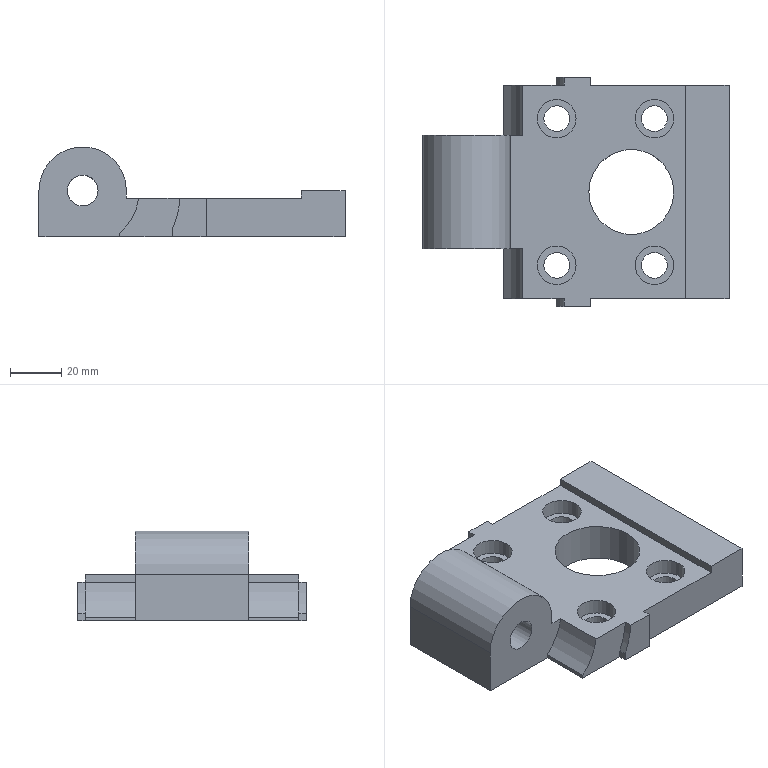Part | NX | features EXTRUDE 11, CBORE_HOLE 4, DATUM_CSYS 4, SKETCH 3, HOLE PACKAGE 1 | 1 solid | 40 faces | box 119 x 89 x 35 mm | volume 132113 mm3 | plane 25 | cylinder 15 | commonest cylinder face diameters 10 x4 15 x4 44 x2 76 x2 12 x1 33 x1
STEP:
#1=CARTESIAN_POINT('',(51.049,70.,15.));
#2=VERTEX_POINT('',#1);
#3=CARTESIAN_POINT('',(58.549,70.,15.));
#4=DIRECTION('',(0.,0.,-1.));
#5=DIRECTION('',(-1.,0.,0.));
#6=AXIS2_PLACEMENT_3D('',#3,#4,#5);
#7=CIRCLE('',#6,7.5);
#8=EDGE_CURVE('',#2,#2,#7,.T.);
#9=ORIENTED_EDGE('',*,*,#8,.T.);
#10=EDGE_LOOP('',(#9));
#11=FACE_BOUND('',#10,.T.);
#12=CARTESIAN_POINT('',(51.049,13.,15.));
#13=VERTEX_POINT('',#12);
#14=CARTESIAN_POINT('',(58.549,13.,15.));
#15=DIRECTION('',(0.,0.,-1.));
#16=DIRECTION('',(-1.,0.,0.));
#17=AXIS2_PLACEMENT_3D('',#14,#15,#16);
#18=CIRCLE('',#17,7.5);
#19=EDGE_CURVE('',#13,#13,#18,.T.);
#20=ORIENTED_EDGE('',*,*,#19,.T.);
#21=EDGE_LOOP('',(#20));
#22=FACE_BOUND('',#21,.T.);
#23=CARTESIAN_POINT('',(13.049,70.,15.));
#24=VERTEX_POINT('',#23);
#25=CARTESIAN_POINT('',(20.549,70.,15.));
#26=DIRECTION('',(0.,0.,-1.));
#27=DIRECTION('',(-1.,0.,0.));
#28=AXIS2_PLACEMENT_3D('',#25,#26,#27);
#29=CIRCLE('',#28,7.5);
#30=EDGE_CURVE('',#24,#24,#29,.T.);
#31=ORIENTED_EDGE('',*,*,#30,.T.);
#32=EDGE_LOOP('',(#31));
#33=FACE_BOUND('',#32,.T.);
#34=CARTESIAN_POINT('',(13.049,13.,15.));
#35=VERTEX_POINT('',#34);
#36=CARTESIAN_POINT('',(20.549,13.,15.));
#37=DIRECTION('',(0.,0.,-1.));
#38=DIRECTION('',(-1.,0.,0.));
#39=AXIS2_PLACEMENT_3D('',#36,#37,#38);
#40=CIRCLE('',#39,7.5);
#41=EDGE_CURVE('',#35,#35,#40,.T.);
#42=ORIENTED_EDGE('',*,*,#41,.T.);
#43=EDGE_LOOP('',(#42));
#44=FACE_BOUND('',#43,.T.);
#45=CARTESIAN_POINT('',(23.43,83.,15.));
#46=VERTEX_POINT('',#45);
#47=CARTESIAN_POINT('',(23.43,86.,15.));
#48=VERTEX_POINT('',#47);
#49=CARTESIAN_POINT('',(23.43,91.5,15.));
#50=DIRECTION('',(0.,-1.,0.));
#51=VECTOR('',#50,1000.);
#52=LINE('',#49,#51);
#53=EDGE_CURVE('',#46,#48,#52,.F.);
#54=ORIENTED_EDGE('',*,*,#53,.F.);
#55=CARTESIAN_POINT('',(7.343,83.,15.));
#56=VERTEX_POINT('',#55);
#57=CARTESIAN_POINT('',(20.342,83.,15.));
#58=DIRECTION('',(-1.,0.,0.));
#59=VECTOR('',#58,1000.);
#60=LINE('',#57,#59);
#61=EDGE_CURVE('',#46,#56,#60,.T.);
#62=ORIENTED_EDGE('',*,*,#61,.T.);
#63=CARTESIAN_POINT('',(7.343,63.5,15.));
#64=VERTEX_POINT('',#63);
#65=CARTESIAN_POINT('',(7.343,91.5,15.));
#66=DIRECTION('',(0.,-1.,0.));
#67=VECTOR('',#66,1000.);
#68=LINE('',#65,#67);
#69=EDGE_CURVE('',#56,#64,#68,.T.);
#70=ORIENTED_EDGE('',*,*,#69,.T.);
#71=CARTESIAN_POINT('',(2.549,63.5,15.));
#72=VERTEX_POINT('',#71);
#73=CARTESIAN_POINT('',(5.549,63.5,15.));
#74=DIRECTION('',(-1.,0.,0.));
#75=VECTOR('',#74,1000.);
#76=LINE('',#73,#75);
#77=EDGE_CURVE('',#64,#72,#76,.T.);
#78=ORIENTED_EDGE('',*,*,#77,.T.);
#79=CARTESIAN_POINT('',(2.549,19.5,15.));
#80=VERTEX_POINT('',#79);
#81=CARTESIAN_POINT('',(2.549,63.5,15.));
#82=DIRECTION('',(0.,-1.,0.));
#83=VECTOR('',#82,1000.);
#84=LINE('',#81,#83);
#85=EDGE_CURVE('',#72,#80,#84,.T.);
#86=ORIENTED_EDGE('',*,*,#85,.T.);
#87=CARTESIAN_POINT('',(7.343,19.5,15.));
#88=VERTEX_POINT('',#87);
#89=CARTESIAN_POINT('',(2.549,19.5,15.));
#90=DIRECTION('',(1.,0.,0.));
#91=VECTOR('',#90,1000.);
#92=LINE('',#89,#91);
#93=EDGE_CURVE('',#80,#88,#92,.T.);
#94=ORIENTED_EDGE('',*,*,#93,.T.);
#95=CARTESIAN_POINT('',(7.343,0.,15.));
#96=VERTEX_POINT('',#95);
#97=CARTESIAN_POINT('',(7.343,-121.5,15.));
#98=DIRECTION('',(0.,1.,0.));
#99=VECTOR('',#98,1000.);
#100=LINE('',#97,#99);
#101=EDGE_CURVE('',#88,#96,#100,.F.);
#102=ORIENTED_EDGE('',*,*,#101,.T.);
#103=CARTESIAN_POINT('',(23.43,0.,15.));
#104=VERTEX_POINT('',#103);
#105=CARTESIAN_POINT('',(5.549,0.,15.));
#106=DIRECTION('',(1.,0.,0.));
#107=VECTOR('',#106,1000.);
#108=LINE('',#105,#107);
#109=EDGE_CURVE('',#96,#104,#108,.T.);
#110=ORIENTED_EDGE('',*,*,#109,.T.);
#111=CARTESIAN_POINT('',(23.43,-3.,15.));
#112=VERTEX_POINT('',#111);
#113=CARTESIAN_POINT('',(23.43,-52.5,15.));
#114=DIRECTION('',(0.,1.,0.));
#115=VECTOR('',#114,1000.);
#116=LINE('',#113,#115);
#117=EDGE_CURVE('',#112,#104,#116,.T.);
#118=ORIENTED_EDGE('',*,*,#117,.F.);
#119=CARTESIAN_POINT('',(33.549,-3.,15.));
#120=VERTEX_POINT('',#119);
#121=CARTESIAN_POINT('',(20.342,-3.,15.));
#122=DIRECTION('',(1.,0.,0.));
#123=VECTOR('',#122,1000.);
#124=LINE('',#121,#123);
#125=EDGE_CURVE('',#112,#120,#124,.T.);
#126=ORIENTED_EDGE('',*,*,#125,.T.);
#127=CARTESIAN_POINT('',(33.549,0.,15.));
#128=VERTEX_POINT('',#127);
#129=CARTESIAN_POINT('',(33.549,-3.,15.));
#130=DIRECTION('',(0.,1.,0.));
#131=VECTOR('',#130,1000.);
#132=LINE('',#129,#131);
#133=EDGE_CURVE('',#120,#128,#132,.T.);
#134=ORIENTED_EDGE('',*,*,#133,.T.);
#135=CARTESIAN_POINT('',(70.549,0.,15.));
#136=VERTEX_POINT('',#135);
#137=CARTESIAN_POINT('',(33.549,0.,15.));
#138=DIRECTION('',(1.,0.,0.));
#139=VECTOR('',#138,1000.);
#140=LINE('',#137,#139);
#141=EDGE_CURVE('',#128,#136,#140,.T.);
#142=ORIENTED_EDGE('',*,*,#141,.T.);
#143=CARTESIAN_POINT('',(70.549,83.,15.));
#144=VERTEX_POINT('',#143);
#145=CARTESIAN_POINT('',(70.549,0.,15.));
#146=DIRECTION('',(0.,1.,0.));
#147=VECTOR('',#146,1000.);
#148=LINE('',#145,#147);
#149=EDGE_CURVE('',#136,#144,#148,.T.);
#150=ORIENTED_EDGE('',*,*,#149,.T.);
#151=CARTESIAN_POINT('',(33.549,83.,15.));
#152=VERTEX_POINT('',#151);
#153=CARTESIAN_POINT('',(70.549,83.,15.));
#154=DIRECTION('',(-1.,0.,0.));
#155=VECTOR('',#154,1000.);
#156=LINE('',#153,#155);
#157=EDGE_CURVE('',#144,#152,#156,.T.);
#158=ORIENTED_EDGE('',*,*,#157,.T.);
#159=CARTESIAN_POINT('',(33.549,86.,15.));
#160=VERTEX_POINT('',#159);
#161=CARTESIAN_POINT('',(33.549,83.,15.));
#162=DIRECTION('',(0.,1.,0.));
#163=VECTOR('',#162,1000.);
#164=LINE('',#161,#163);
#165=EDGE_CURVE('',#152,#160,#164,.T.);
#166=ORIENTED_EDGE('',*,*,#165,.T.);
#167=CARTESIAN_POINT('',(33.549,86.,15.));
#168=DIRECTION('',(-1.,0.,0.));
#169=VECTOR('',#168,1000.);
#170=LINE('',#167,#169);
#171=EDGE_CURVE('',#160,#48,#170,.T.);
#172=ORIENTED_EDGE('',*,*,#171,.T.);
#173=EDGE_LOOP('',(#54,#62,#70,#78,#86,#94,#102,#110,#118,#126,#134,#142,#150,#158,#166,#172));
#174=FACE_BOUND('',#173,.T.);
#175=CARTESIAN_POINT('',(66.049,41.5,15.));
#176=VERTEX_POINT('',#175);
#177=CARTESIAN_POINT('',(49.549,41.5,15.));
#178=DIRECTION('',(0.,0.,1.));
#179=DIRECTION('',(1.,0.,0.));
#180=AXIS2_PLACEMENT_3D('',#177,#178,#179);
#181=CIRCLE('',#180,16.5);
#182=EDGE_CURVE('',#176,#176,#181,.T.);
#183=ORIENTED_EDGE('',*,*,#182,.F.);
#184=EDGE_LOOP('',(#183));
#185=FACE_BOUND('',#184,.T.);
#186=CARTESIAN_POINT('',(49.549,41.5,15.));
#187=DIRECTION('',(0.,0.,1.));
#188=DIRECTION('',(1.,0.,0.));
#189=AXIS2_PLACEMENT_3D('',#186,#187,#188);
#190=PLANE('',#189);
#191=ADVANCED_FACE('',(#11,#22,#33,#44,#174,#185),#190,.T.);
#192=CARTESIAN_POINT('',(0.,83.,1.412));
#193=VERTEX_POINT('',#192);
#194=CARTESIAN_POINT('',(0.,63.5,1.412));
#195=VERTEX_POINT('',#194);
#196=CARTESIAN_POINT('',(0.,91.5,1.412));
#197=DIRECTION('',(0.,-1.,0.));
#198=VECTOR('',#197,1000.);
#199=LINE('',#196,#198);
#200=EDGE_CURVE('',#193,#195,#199,.T.);
#201=ORIENTED_EDGE('',*,*,#200,.F.);
#202=CARTESIAN_POINT('',(0.,83.,0.));
#203=VERTEX_POINT('',#202);
#204=CARTESIAN_POINT('',(0.,83.,35.));
#205=DIRECTION('',(0.,0.,-1.));
#206=VECTOR('',#205,1000.);
#207=LINE('',#204,#206);
#208=EDGE_CURVE('',#193,#203,#207,.T.);
#209=ORIENTED_EDGE('',*,*,#208,.T.);
#210=CARTESIAN_POINT('',(0.,63.5,0.));
#211=VERTEX_POINT('',#210);
#212=CARTESIAN_POINT('',(0.,83.,0.));
#213=DIRECTION('',(0.,-1.,0.));
#214=VECTOR('',#213,1000.);
#215=LINE('',#212,#214);
#216=EDGE_CURVE('',#203,#211,#215,.T.);
#217=ORIENTED_EDGE('',*,*,#216,.T.);
#218=CARTESIAN_POINT('',(0.,63.5,35.));
#219=DIRECTION('',(0.,0.,-1.));
#220=VECTOR('',#219,1000.);
#221=LINE('',#218,#220);
#222=EDGE_CURVE('',#195,#211,#221,.T.);
#223=ORIENTED_EDGE('',*,*,#222,.F.);
#224=EDGE_LOOP('',(#201,#209,#217,#223));
#225=FACE_BOUND('',#224,.T.);
#226=CARTESIAN_POINT('',(0.,83.,35.));
#227=DIRECTION('',(1.,0.,0.));
#228=DIRECTION('',(0.,1.,0.));
#229=AXIS2_PLACEMENT_3D('',#226,#227,#228);
#230=PLANE('',#229);
#231=ADVANCED_FACE('',(#225),#230,.F.);
#232=CARTESIAN_POINT('',(2.549,19.5,18.));
#233=VERTEX_POINT('',#232);
#234=CARTESIAN_POINT('',(2.549,63.5,18.));
#235=VERTEX_POINT('',#234);
#236=CARTESIAN_POINT('',(2.549,-121.5,18.));
#237=DIRECTION('',(0.,1.,0.));
#238=VECTOR('',#237,1000.);
#239=LINE('',#236,#238);
#240=EDGE_CURVE('',#233,#235,#239,.T.);
#241=ORIENTED_EDGE('',*,*,#240,.T.);
#242=CARTESIAN_POINT('',(-31.451,63.5,18.));
#243=VERTEX_POINT('',#242);
#244=CARTESIAN_POINT('',(-14.451,63.5,18.));
#245=DIRECTION('',(0.,-1.,0.));
#246=DIRECTION('',(0.,0.,-1.));
#247=AXIS2_PLACEMENT_3D('',#244,#245,#246);
#248=CIRCLE('',#247,17.);
#249=EDGE_CURVE('',#235,#243,#248,.T.);
#250=ORIENTED_EDGE('',*,*,#249,.T.);
#251=CARTESIAN_POINT('',(-31.451,19.5,18.));
#252=VERTEX_POINT('',#251);
#253=CARTESIAN_POINT('',(-31.451,-121.5,18.));
#254=DIRECTION('',(0.,1.,0.));
#255=VECTOR('',#254,1000.);
#256=LINE('',#253,#255);
#257=EDGE_CURVE('',#252,#243,#256,.T.);
#258=ORIENTED_EDGE('',*,*,#257,.F.);
#259=CARTESIAN_POINT('',(-14.451,19.5,18.));
#260=DIRECTION('',(0.,1.,0.));
#261=DIRECTION('',(-1.,0.,0.));
#262=AXIS2_PLACEMENT_3D('',#259,#260,#261);
#263=CIRCLE('',#262,17.);
#264=EDGE_CURVE('',#252,#233,#263,.T.);
#265=ORIENTED_EDGE('',*,*,#264,.T.);
#266=EDGE_LOOP('',(#241,#250,#258,#265));
#267=FACE_BOUND('',#266,.T.);
#268=CARTESIAN_POINT('',(-14.451,-121.5,18.));
#269=DIRECTION('',(0.,1.,0.));
#270=DIRECTION('',(0.,0.,1.));
#271=AXIS2_PLACEMENT_3D('',#268,#269,#270);
#272=CYLINDRICAL_SURFACE('',#271,17.);
#273=ADVANCED_FACE('',(#267),#272,.T.);
#274=CARTESIAN_POINT('',(0.,19.5,1.412));
#275=VERTEX_POINT('',#274);
#276=CARTESIAN_POINT('',(0.,0.,1.412));
#277=VERTEX_POINT('',#276);
#278=CARTESIAN_POINT('',(0.,-121.5,1.412));
#279=DIRECTION('',(0.,1.,0.));
#280=VECTOR('',#279,1000.);
#281=LINE('',#278,#280);
#282=EDGE_CURVE('',#275,#277,#281,.F.);
#283=ORIENTED_EDGE('',*,*,#282,.F.);
#284=CARTESIAN_POINT('',(0.,19.5,0.));
#285=VERTEX_POINT('',#284);
#286=CARTESIAN_POINT('',(0.,19.5,35.));
#287=DIRECTION('',(0.,0.,-1.));
#288=VECTOR('',#287,1000.);
#289=LINE('',#286,#288);
#290=EDGE_CURVE('',#275,#285,#289,.T.);
#291=ORIENTED_EDGE('',*,*,#290,.T.);
#292=CARTESIAN_POINT('',(0.,0.,0.));
#293=VERTEX_POINT('',#292);
#294=CARTESIAN_POINT('',(0.,19.5,0.));
#295=DIRECTION('',(0.,-1.,0.));
#296=VECTOR('',#295,1000.);
#297=LINE('',#294,#296);
#298=EDGE_CURVE('',#285,#293,#297,.T.);
#299=ORIENTED_EDGE('',*,*,#298,.T.);
#300=CARTESIAN_POINT('',(0.,0.,35.));
#301=DIRECTION('',(0.,0.,-1.));
#302=VECTOR('',#301,1000.);
#303=LINE('',#300,#302);
#304=EDGE_CURVE('',#277,#293,#303,.T.);
#305=ORIENTED_EDGE('',*,*,#304,.F.);
#306=EDGE_LOOP('',(#283,#291,#299,#305));
#307=FACE_BOUND('',#306,.T.);
#308=CARTESIAN_POINT('',(0.,19.5,35.));
#309=DIRECTION('',(1.,0.,0.));
#310=DIRECTION('',(0.,1.,0.));
#311=AXIS2_PLACEMENT_3D('',#308,#309,#310);
#312=PLANE('',#311);
#313=ADVANCED_FACE('',(#307),#312,.F.);
#314=CARTESIAN_POINT('',(20.342,0.,2.722));
#315=VERTEX_POINT('',#314);
#316=CARTESIAN_POINT('',(20.342,0.,0.));
#317=VERTEX_POINT('',#316);
#318=CARTESIAN_POINT('',(20.342,0.,15.));
#319=DIRECTION('',(0.,0.,-1.));
#320=VECTOR('',#319,1000.);
#321=LINE('',#318,#320);
#322=EDGE_CURVE('',#315,#317,#321,.T.);
#323=ORIENTED_EDGE('',*,*,#322,.F.);
#324=CARTESIAN_POINT('',(-14.451,0.,18.));
#325=DIRECTION('',(0.,1.,0.));
#326=DIRECTION('',(1.,0.,0.));
#327=AXIS2_PLACEMENT_3D('',#324,#325,#326);
#328=CIRCLE('',#327,38.);
#329=EDGE_CURVE('',#104,#315,#328,.T.);
#330=ORIENTED_EDGE('',*,*,#329,.F.);
#331=ORIENTED_EDGE('',*,*,#109,.F.);
#332=CARTESIAN_POINT('',(-14.451,0.,18.));
#333=DIRECTION('',(0.,1.,0.));
#334=DIRECTION('',(-1.,0.,0.));
#335=AXIS2_PLACEMENT_3D('',#332,#333,#334);
#336=CIRCLE('',#335,22.);
#337=EDGE_CURVE('',#277,#96,#336,.F.);
#338=ORIENTED_EDGE('',*,*,#337,.F.);
#339=ORIENTED_EDGE('',*,*,#304,.T.);
#340=CARTESIAN_POINT('',(0.,0.,0.));
#341=DIRECTION('',(1.,0.,0.));
#342=VECTOR('',#341,1000.);
#343=LINE('',#340,#342);
#344=EDGE_CURVE('',#293,#317,#343,.T.);
#345=ORIENTED_EDGE('',*,*,#344,.T.);
#346=EDGE_LOOP('',(#323,#330,#331,#338,#339,#345));
#347=FACE_BOUND('',#346,.T.);
#348=CARTESIAN_POINT('',(0.,0.,35.));
#349=DIRECTION('',(0.,1.,0.));
#350=DIRECTION('',(-1.,0.,0.));
#351=AXIS2_PLACEMENT_3D('',#348,#349,#350);
#352=PLANE('',#351);
#353=ADVANCED_FACE('',(#347),#352,.F.);
#354=ORIENTED_EDGE('',*,*,#240,.F.);
#355=CARTESIAN_POINT('',(2.549,19.5,35.));
#356=DIRECTION('',(0.,0.,-1.));
#357=VECTOR('',#356,1000.);
#358=LINE('',#355,#357);
#359=EDGE_CURVE('',#233,#80,#358,.T.);
#360=ORIENTED_EDGE('',*,*,#359,.T.);
#361=ORIENTED_EDGE('',*,*,#85,.F.);
#362=CARTESIAN_POINT('',(2.549,63.5,35.));
#363=DIRECTION('',(0.,0.,-1.));
#364=VECTOR('',#363,1000.);
#365=LINE('',#362,#364);
#366=EDGE_CURVE('',#235,#72,#365,.T.);
#367=ORIENTED_EDGE('',*,*,#366,.F.);
#368=EDGE_LOOP('',(#354,#360,#361,#367));
#369=FACE_BOUND('',#368,.T.);
#370=CARTESIAN_POINT('',(2.549,19.5,35.));
#371=DIRECTION('',(-1.,0.,0.));
#372=DIRECTION('',(0.,-1.,0.));
#373=AXIS2_PLACEMENT_3D('',#370,#371,#372);
#374=PLANE('',#373);
#375=ADVANCED_FACE('',(#369),#374,.F.);
#376=CARTESIAN_POINT('',(-8.451,19.5,18.));
#377=VERTEX_POINT('',#376);
#378=CARTESIAN_POINT('',(-14.451,19.5,18.));
#379=DIRECTION('',(0.,-1.,0.));
#380=DIRECTION('',(1.,0.,0.));
#381=AXIS2_PLACEMENT_3D('',#378,#379,#380);
#382=CIRCLE('',#381,6.);
#383=EDGE_CURVE('',#377,#377,#382,.T.);
#384=ORIENTED_EDGE('',*,*,#383,.F.);
#385=EDGE_LOOP('',(#384));
#386=FACE_BOUND('',#385,.T.);
#387=ORIENTED_EDGE('',*,*,#359,.F.);
#388=ORIENTED_EDGE('',*,*,#264,.F.);
#389=CARTESIAN_POINT('',(-31.451,19.5,0.));
#390=VERTEX_POINT('',#389);
#391=CARTESIAN_POINT('',(-31.451,19.5,35.));
#392=DIRECTION('',(0.,0.,-1.));
#393=VECTOR('',#392,1000.);
#394=LINE('',#391,#393);
#395=EDGE_CURVE('',#252,#390,#394,.T.);
#396=ORIENTED_EDGE('',*,*,#395,.T.);
#397=CARTESIAN_POINT('',(-31.451,19.5,0.));
#398=DIRECTION('',(1.,0.,0.));
#399=VECTOR('',#398,1000.);
#400=LINE('',#397,#399);
#401=EDGE_CURVE('',#390,#285,#400,.T.);
#402=ORIENTED_EDGE('',*,*,#401,.T.);
#403=ORIENTED_EDGE('',*,*,#290,.F.);
#404=CARTESIAN_POINT('',(-14.451,19.5,18.));
#405=DIRECTION('',(0.,-1.,0.));
#406=DIRECTION('',(1.,0.,0.));
#407=AXIS2_PLACEMENT_3D('',#404,#405,#406);
#408=CIRCLE('',#407,22.);
#409=EDGE_CURVE('',#275,#88,#408,.T.);
#410=ORIENTED_EDGE('',*,*,#409,.T.);
#411=ORIENTED_EDGE('',*,*,#93,.F.);
#412=EDGE_LOOP('',(#387,#388,#396,#402,#403,#410,#411));
#413=FACE_BOUND('',#412,.T.);
#414=CARTESIAN_POINT('',(-31.451,19.5,35.));
#415=DIRECTION('',(0.,1.,0.));
#416=DIRECTION('',(-1.,0.,0.));
#417=AXIS2_PLACEMENT_3D('',#414,#415,#416);
#418=PLANE('',#417);
#419=ADVANCED_FACE('',(#386,#413),#418,.F.);
#420=CARTESIAN_POINT('',(20.342,83.,0.));
#421=VERTEX_POINT('',#420);
#422=CARTESIAN_POINT('',(5.549,83.,0.));
#423=DIRECTION('',(-1.,0.,0.));
#424=VECTOR('',#423,1000.);
#425=LINE('',#422,#424);
#426=EDGE_CURVE('',#421,#203,#425,.T.);
#427=ORIENTED_EDGE('',*,*,#426,.T.);
#428=ORIENTED_EDGE('',*,*,#208,.F.);
#429=CARTESIAN_POINT('',(-14.451,83.,18.));
#430=DIRECTION('',(0.,-1.,0.));
#431=DIRECTION('',(0.,0.,-1.));
#432=AXIS2_PLACEMENT_3D('',#429,#430,#431);
#433=CIRCLE('',#432,22.);
#434=EDGE_CURVE('',#56,#193,#433,.F.);
#435=ORIENTED_EDGE('',*,*,#434,.F.);
#436=ORIENTED_EDGE('',*,*,#61,.F.);
#437=CARTESIAN_POINT('',(20.342,83.,2.722));
#438=VERTEX_POINT('',#437);
#439=CARTESIAN_POINT('',(-14.451,83.,18.));
#440=DIRECTION('',(0.,-1.,0.));
#441=DIRECTION('',(1.,0.,0.));
#442=AXIS2_PLACEMENT_3D('',#439,#440,#441);
#443=CIRCLE('',#442,38.);
#444=EDGE_CURVE('',#438,#46,#443,.T.);
#445=ORIENTED_EDGE('',*,*,#444,.F.);
#446=CARTESIAN_POINT('',(20.342,83.,15.));
#447=DIRECTION('',(0.,0.,-1.));
#448=VECTOR('',#447,1000.);
#449=LINE('',#446,#448);
#450=EDGE_CURVE('',#438,#421,#449,.T.);
#451=ORIENTED_EDGE('',*,*,#450,.T.);
#452=EDGE_LOOP('',(#427,#428,#435,#436,#445,#451));
#453=FACE_BOUND('',#452,.T.);
#454=CARTESIAN_POINT('',(5.549,83.,35.));
#455=DIRECTION('',(0.,-1.,0.));
#456=DIRECTION('',(0.,0.,-1.));
#457=AXIS2_PLACEMENT_3D('',#454,#455,#456);
#458=PLANE('',#457);
#459=ADVANCED_FACE('',(#453),#458,.F.);
#460=CARTESIAN_POINT('',(-14.451,63.5,12.));
#461=VERTEX_POINT('',#460);
#462=CARTESIAN_POINT('',(-14.451,63.5,18.));
#463=DIRECTION('',(0.,-1.,0.));
#464=DIRECTION('',(0.,0.,-1.));
#465=AXIS2_PLACEMENT_3D('',#462,#463,#464);
#466=CIRCLE('',#465,6.);
#467=EDGE_CURVE('',#461,#461,#466,.T.);
#468=ORIENTED_EDGE('',*,*,#467,.T.);
#469=EDGE_LOOP('',(#468));
#470=FACE_BOUND('',#469,.T.);
#471=CARTESIAN_POINT('',(-14.451,63.5,18.));
#472=DIRECTION('',(0.,1.,0.));
#473=DIRECTION('',(1.,0.,0.));
#474=AXIS2_PLACEMENT_3D('',#471,#472,#473);
#475=CIRCLE('',#474,22.);
#476=EDGE_CURVE('',#64,#195,#475,.T.);
#477=ORIENTED_EDGE('',*,*,#476,.T.);
#478=ORIENTED_EDGE('',*,*,#222,.T.);
#479=CARTESIAN_POINT('',(-31.451,63.5,0.));
#480=VERTEX_POINT('',#479);
#481=CARTESIAN_POINT('',(0.,63.5,0.));
#482=DIRECTION('',(-1.,0.,0.));
#483=VECTOR('',#482,1000.);
#484=LINE('',#481,#483);
#485=EDGE_CURVE('',#211,#480,#484,.T.);
#486=ORIENTED_EDGE('',*,*,#485,.T.);
#487=CARTESIAN_POINT('',(-31.451,63.5,35.));
#488=DIRECTION('',(0.,0.,-1.));
#489=VECTOR('',#488,1000.);
#490=LINE('',#487,#489);
#491=EDGE_CURVE('',#243,#480,#490,.T.);
#492=ORIENTED_EDGE('',*,*,#491,.F.);
#493=ORIENTED_EDGE('',*,*,#249,.F.);
#494=ORIENTED_EDGE('',*,*,#366,.T.);
#495=ORIENTED_EDGE('',*,*,#77,.F.);
#496=EDGE_LOOP('',(#477,#478,#486,#492,#493,#494,#495));
#497=FACE_BOUND('',#496,.T.);
#498=CARTESIAN_POINT('',(0.,63.5,35.));
#499=DIRECTION('',(0.,-1.,0.));
#500=DIRECTION('',(0.,0.,-1.));
#501=AXIS2_PLACEMENT_3D('',#498,#499,#500);
#502=PLANE('',#501);
#503=ADVANCED_FACE('',(#470,#497),#502,.F.);
#504=ORIENTED_EDGE('',*,*,#395,.F.);
#505=ORIENTED_EDGE('',*,*,#257,.T.);
#506=ORIENTED_EDGE('',*,*,#491,.T.);
#507=CARTESIAN_POINT('',(-31.451,63.5,0.));
#508=DIRECTION('',(0.,-1.,0.));
#509=VECTOR('',#508,1000.);
#510=LINE('',#507,#509);
#511=EDGE_CURVE('',#480,#390,#510,.T.);
#512=ORIENTED_EDGE('',*,*,#511,.T.);
#513=EDGE_LOOP('',(#504,#505,#506,#512));
#514=FACE_BOUND('',#513,.T.);
#515=CARTESIAN_POINT('',(-31.451,63.5,35.));
#516=DIRECTION('',(1.,0.,0.));
#517=DIRECTION('',(0.,1.,0.));
#518=AXIS2_PLACEMENT_3D('',#515,#516,#517);
#519=PLANE('',#518);
#520=ADVANCED_FACE('',(#514),#519,.F.);
#521=CARTESIAN_POINT('',(63.549,70.,0.));
#522=VERTEX_POINT('',#521);
#523=CARTESIAN_POINT('',(58.549,70.,0.));
#524=DIRECTION('',(0.,0.,1.));
#525=DIRECTION('',(1.,0.,0.));
#526=AXIS2_PLACEMENT_3D('',#523,#524,#525);
#527=CIRCLE('',#526,5.);
#528=EDGE_CURVE('',#522,#522,#527,.T.);
#529=ORIENTED_EDGE('',*,*,#528,.T.);
#530=EDGE_LOOP('',(#529));
#531=FACE_BOUND('',#530,.T.);
#532=CARTESIAN_POINT('',(63.549,13.,0.));
#533=VERTEX_POINT('',#532);
#534=CARTESIAN_POINT('',(58.549,13.,0.));
#535=DIRECTION('',(0.,0.,1.));
#536=DIRECTION('',(1.,0.,0.));
#537=AXIS2_PLACEMENT_3D('',#534,#535,#536);
#538=CIRCLE('',#537,5.);
#539=EDGE_CURVE('',#533,#533,#538,.T.);
#540=ORIENTED_EDGE('',*,*,#539,.T.);
#541=EDGE_LOOP('',(#540));
#542=FACE_BOUND('',#541,.T.);
#543=CARTESIAN_POINT('',(25.549,70.,0.));
#544=VERTEX_POINT('',#543);
#545=CARTESIAN_POINT('',(20.549,70.,0.));
#546=DIRECTION('',(0.,0.,1.));
#547=DIRECTION('',(1.,0.,0.));
#548=AXIS2_PLACEMENT_3D('',#545,#546,#547);
#549=CIRCLE('',#548,5.);
#550=EDGE_CURVE('',#544,#544,#549,.T.);
#551=ORIENTED_EDGE('',*,*,#550,.T.);
#552=EDGE_LOOP('',(#551));
#553=FACE_BOUND('',#552,.T.);
#554=CARTESIAN_POINT('',(25.549,13.,0.));
#555=VERTEX_POINT('',#554);
#556=CARTESIAN_POINT('',(20.549,13.,0.));
#557=DIRECTION('',(0.,0.,1.));
#558=DIRECTION('',(1.,0.,0.));
#559=AXIS2_PLACEMENT_3D('',#556,#557,#558);
#560=CIRCLE('',#559,5.);
#561=EDGE_CURVE('',#555,#555,#560,.T.);
#562=ORIENTED_EDGE('',*,*,#561,.T.);
#563=EDGE_LOOP('',(#562));
#564=FACE_BOUND('',#563,.T.);
#565=ORIENTED_EDGE('',*,*,#511,.F.);
#566=ORIENTED_EDGE('',*,*,#485,.F.);
#567=ORIENTED_EDGE('',*,*,#216,.F.);
#568=ORIENTED_EDGE('',*,*,#426,.F.);
#569=CARTESIAN_POINT('',(20.342,86.,0.));
#570=VERTEX_POINT('',#569);
#571=CARTESIAN_POINT('',(20.342,86.,0.));
#572=DIRECTION('',(0.,-1.,0.));
#573=VECTOR('',#572,1000.);
#574=LINE('',#571,#573);
#575=EDGE_CURVE('',#570,#421,#574,.T.);
#576=ORIENTED_EDGE('',*,*,#575,.F.);
#577=CARTESIAN_POINT('',(33.549,86.,0.));
#578=VERTEX_POINT('',#577);
#579=CARTESIAN_POINT('',(23.549,86.,0.));
#580=DIRECTION('',(-1.,0.,0.));
#581=VECTOR('',#580,1000.);
#582=LINE('',#579,#581);
#583=EDGE_CURVE('',#578,#570,#582,.T.);
#584=ORIENTED_EDGE('',*,*,#583,.F.);
#585=CARTESIAN_POINT('',(33.549,83.,0.));
#586=VERTEX_POINT('',#585);
#587=CARTESIAN_POINT('',(33.549,83.,0.));
#588=DIRECTION('',(0.,1.,0.));
#589=VECTOR('',#588,1000.);
#590=LINE('',#587,#589);
#591=EDGE_CURVE('',#586,#578,#590,.T.);
#592=ORIENTED_EDGE('',*,*,#591,.F.);
#593=CARTESIAN_POINT('',(87.549,83.,0.));
#594=VERTEX_POINT('',#593);
#595=CARTESIAN_POINT('',(70.549,83.,0.));
#596=DIRECTION('',(-1.,0.,0.));
#597=VECTOR('',#596,1000.);
#598=LINE('',#595,#597);
#599=EDGE_CURVE('',#594,#586,#598,.T.);
#600=ORIENTED_EDGE('',*,*,#599,.F.);
#601=CARTESIAN_POINT('',(87.549,0.,0.));
#602=VERTEX_POINT('',#601);
#603=CARTESIAN_POINT('',(87.549,0.,0.));
#604=DIRECTION('',(0.,1.,0.));
#605=VECTOR('',#604,1000.);
#606=LINE('',#603,#605);
#607=EDGE_CURVE('',#602,#594,#606,.T.);
#608=ORIENTED_EDGE('',*,*,#607,.F.);
#609=CARTESIAN_POINT('',(33.549,0.,0.));
#610=VERTEX_POINT('',#609);
#611=CARTESIAN_POINT('',(33.549,0.,0.));
#612=DIRECTION('',(1.,0.,0.));
#613=VECTOR('',#612,1000.);
#614=LINE('',#611,#613);
#615=EDGE_CURVE('',#610,#602,#614,.T.);
#616=ORIENTED_EDGE('',*,*,#615,.F.);
#617=CARTESIAN_POINT('',(33.549,-3.,0.));
#618=VERTEX_POINT('',#617);
#619=CARTESIAN_POINT('',(33.549,-3.,0.));
#620=DIRECTION('',(0.,1.,0.));
#621=VECTOR('',#620,1000.);
#622=LINE('',#619,#621);
#623=EDGE_CURVE('',#618,#610,#622,.T.);
#624=ORIENTED_EDGE('',*,*,#623,.F.);
#625=CARTESIAN_POINT('',(20.342,-3.,0.));
#626=VERTEX_POINT('',#625);
#627=CARTESIAN_POINT('',(23.549,-3.,0.));
#628=DIRECTION('',(1.,0.,0.));
#629=VECTOR('',#628,1000.);
#630=LINE('',#627,#629);
#631=EDGE_CURVE('',#626,#618,#630,.T.);
#632=ORIENTED_EDGE('',*,*,#631,.F.);
#633=CARTESIAN_POINT('',(20.342,0.,0.));
#634=DIRECTION('',(0.,-1.,0.));
#635=VECTOR('',#634,1000.);
#636=LINE('',#633,#635);
#637=EDGE_CURVE('',#317,#626,#636,.T.);
#638=ORIENTED_EDGE('',*,*,#637,.F.);
#639=ORIENTED_EDGE('',*,*,#344,.F.);
#640=ORIENTED_EDGE('',*,*,#298,.F.);
#641=ORIENTED_EDGE('',*,*,#401,.F.);
#642=EDGE_LOOP('',(#565,#566,#567,#568,#576,#584,#592,#600,#608,#616,#624,#632,#638,#639,#640,#641));
#643=FACE_BOUND('',#642,.T.);
#644=CARTESIAN_POINT('',(66.049,41.5,0.));
#645=VERTEX_POINT('',#644);
#646=CARTESIAN_POINT('',(49.549,41.5,0.));
#647=DIRECTION('',(0.,0.,1.));
#648=DIRECTION('',(1.,0.,0.));
#649=AXIS2_PLACEMENT_3D('',#646,#647,#648);
#650=CIRCLE('',#649,16.5);
#651=EDGE_CURVE('',#645,#645,#650,.T.);
#652=ORIENTED_EDGE('',*,*,#651,.T.);
#653=EDGE_LOOP('',(#652));
#654=FACE_BOUND('',#653,.T.);
#655=CARTESIAN_POINT('',(0.,0.,0.));
#656=DIRECTION('',(0.,0.,1.));
#657=DIRECTION('',(1.,0.,0.));
#658=AXIS2_PLACEMENT_3D('',#655,#656,#657);
#659=PLANE('',#658);
#660=ADVANCED_FACE('',(#531,#542,#553,#564,#643,#654),#659,.F.);
#661=CARTESIAN_POINT('',(20.342,-3.,2.722));
#662=VERTEX_POINT('',#661);
#663=CARTESIAN_POINT('',(20.342,-3.,15.));
#664=DIRECTION('',(0.,0.,-1.));
#665=VECTOR('',#664,1000.);
#666=LINE('',#663,#665);
#667=EDGE_CURVE('',#662,#626,#666,.T.);
#668=ORIENTED_EDGE('',*,*,#667,.F.);
#669=CARTESIAN_POINT('',(20.342,-52.5,2.722));
#670=DIRECTION('',(0.,1.,0.));
#671=VECTOR('',#670,1000.);
#672=LINE('',#669,#671);
#673=EDGE_CURVE('',#662,#315,#672,.T.);
#674=ORIENTED_EDGE('',*,*,#673,.T.);
#675=ORIENTED_EDGE('',*,*,#322,.T.);
#676=ORIENTED_EDGE('',*,*,#637,.T.);
#677=EDGE_LOOP('',(#668,#674,#675,#676));
#678=FACE_BOUND('',#677,.T.);
#679=CARTESIAN_POINT('',(20.342,0.,15.));
#680=DIRECTION('',(1.,0.,0.));
#681=DIRECTION('',(0.,0.,-1.));
#682=AXIS2_PLACEMENT_3D('',#679,#680,#681);
#683=PLANE('',#682);
#684=ADVANCED_FACE('',(#678),#683,.F.);
#685=ORIENTED_EDGE('',*,*,#125,.F.);
#686=CARTESIAN_POINT('',(-14.451,-3.,18.));
#687=DIRECTION('',(0.,1.,0.));
#688=DIRECTION('',(-1.,0.,0.));
#689=AXIS2_PLACEMENT_3D('',#686,#687,#688);
#690=CIRCLE('',#689,38.);
#691=EDGE_CURVE('',#112,#662,#690,.T.);
#692=ORIENTED_EDGE('',*,*,#691,.T.);
#693=ORIENTED_EDGE('',*,*,#667,.T.);
#694=ORIENTED_EDGE('',*,*,#631,.T.);
#695=CARTESIAN_POINT('',(33.549,-3.,15.));
#696=DIRECTION('',(0.,0.,-1.));
#697=VECTOR('',#696,1000.);
#698=LINE('',#695,#697);
#699=EDGE_CURVE('',#120,#618,#698,.T.);
#700=ORIENTED_EDGE('',*,*,#699,.F.);
#701=EDGE_LOOP('',(#685,#692,#693,#694,#700));
#702=FACE_BOUND('',#701,.T.);
#703=CARTESIAN_POINT('',(23.549,-3.,15.));
#704=DIRECTION('',(0.,1.,0.));
#705=DIRECTION('',(-1.,0.,0.));
#706=AXIS2_PLACEMENT_3D('',#703,#704,#705);
#707=PLANE('',#706);
#708=ADVANCED_FACE('',(#702),#707,.F.);
#709=ORIENTED_EDGE('',*,*,#623,.T.);
#710=CARTESIAN_POINT('',(33.549,0.,15.));
#711=DIRECTION('',(0.,0.,-1.));
#712=VECTOR('',#711,1000.);
#713=LINE('',#710,#712);
#714=EDGE_CURVE('',#128,#610,#713,.T.);
#715=ORIENTED_EDGE('',*,*,#714,.F.);
#716=ORIENTED_EDGE('',*,*,#133,.F.);
#717=ORIENTED_EDGE('',*,*,#699,.T.);
#718=EDGE_LOOP('',(#709,#715,#716,#717));
#719=FACE_BOUND('',#718,.T.);
#720=CARTESIAN_POINT('',(33.549,-3.,15.));
#721=DIRECTION('',(-1.,0.,0.));
#722=DIRECTION('',(0.,-1.,0.));
#723=AXIS2_PLACEMENT_3D('',#720,#721,#722);
#724=PLANE('',#723);
#725=ADVANCED_FACE('',(#719),#724,.F.);
#726=ORIENTED_EDGE('',*,*,#615,.T.);
#727=CARTESIAN_POINT('',(87.549,0.,18.));
#728=VERTEX_POINT('',#727);
#729=CARTESIAN_POINT('',(87.549,0.,18.));
#730=DIRECTION('',(0.,0.,-1.));
#731=VECTOR('',#730,1000.);
#732=LINE('',#729,#731);
#733=EDGE_CURVE('',#728,#602,#732,.T.);
#734=ORIENTED_EDGE('',*,*,#733,.F.);
#735=CARTESIAN_POINT('',(70.549,0.,18.));
#736=VERTEX_POINT('',#735);
#737=CARTESIAN_POINT('',(70.549,0.,18.));
#738=DIRECTION('',(1.,0.,0.));
#739=VECTOR('',#738,1000.);
#740=LINE('',#737,#739);
#741=EDGE_CURVE('',#736,#728,#740,.T.);
#742=ORIENTED_EDGE('',*,*,#741,.F.);
#743=CARTESIAN_POINT('',(70.549,0.,18.));
#744=DIRECTION('',(0.,0.,-1.));
#745=VECTOR('',#744,1000.);
#746=LINE('',#743,#745);
#747=EDGE_CURVE('',#736,#136,#746,.T.);
#748=ORIENTED_EDGE('',*,*,#747,.T.);
#749=ORIENTED_EDGE('',*,*,#141,.F.);
#750=ORIENTED_EDGE('',*,*,#714,.T.);
#751=EDGE_LOOP('',(#726,#734,#742,#748,#749,#750));
#752=FACE_BOUND('',#751,.T.);
#753=CARTESIAN_POINT('',(33.549,0.,15.));
#754=DIRECTION('',(0.,1.,0.));
#755=DIRECTION('',(-1.,0.,0.));
#756=AXIS2_PLACEMENT_3D('',#753,#754,#755);
#757=PLANE('',#756);
#758=ADVANCED_FACE('',(#752),#757,.F.);
#759=ORIENTED_EDGE('',*,*,#599,.T.);
#760=CARTESIAN_POINT('',(33.549,83.,15.));
#761=DIRECTION('',(0.,0.,-1.));
#762=VECTOR('',#761,1000.);
#763=LINE('',#760,#762);
#764=EDGE_CURVE('',#152,#586,#763,.T.);
#765=ORIENTED_EDGE('',*,*,#764,.F.);
#766=ORIENTED_EDGE('',*,*,#157,.F.);
#767=CARTESIAN_POINT('',(70.549,83.,18.));
#768=VERTEX_POINT('',#767);
#769=CARTESIAN_POINT('',(70.549,83.,18.));
#770=DIRECTION('',(0.,0.,-1.));
#771=VECTOR('',#770,1000.);
#772=LINE('',#769,#771);
#773=EDGE_CURVE('',#768,#144,#772,.T.);
#774=ORIENTED_EDGE('',*,*,#773,.F.);
#775=CARTESIAN_POINT('',(87.549,83.,18.));
#776=VERTEX_POINT('',#775);
#777=CARTESIAN_POINT('',(87.549,83.,18.));
#778=DIRECTION('',(-1.,0.,0.));
#779=VECTOR('',#778,1000.);
#780=LINE('',#777,#779);
#781=EDGE_CURVE('',#776,#768,#780,.T.);
#782=ORIENTED_EDGE('',*,*,#781,.F.);
#783=CARTESIAN_POINT('',(87.549,83.,18.));
#784=DIRECTION('',(0.,0.,-1.));
#785=VECTOR('',#784,1000.);
#786=LINE('',#783,#785);
#787=EDGE_CURVE('',#776,#594,#786,.T.);
#788=ORIENTED_EDGE('',*,*,#787,.T.);
#789=EDGE_LOOP('',(#759,#765,#766,#774,#782,#788));
#790=FACE_BOUND('',#789,.T.);
#791=CARTESIAN_POINT('',(70.549,83.,15.));
#792=DIRECTION('',(0.,-1.,0.));
#793=DIRECTION('',(1.,0.,0.));
#794=AXIS2_PLACEMENT_3D('',#791,#792,#793);
#795=PLANE('',#794);
#796=ADVANCED_FACE('',(#790),#795,.F.);
#797=ORIENTED_EDGE('',*,*,#591,.T.);
#798=CARTESIAN_POINT('',(33.549,86.,15.));
#799=DIRECTION('',(0.,0.,-1.));
#800=VECTOR('',#799,1000.);
#801=LINE('',#798,#800);
#802=EDGE_CURVE('',#160,#578,#801,.T.);
#803=ORIENTED_EDGE('',*,*,#802,.F.);
#804=ORIENTED_EDGE('',*,*,#165,.F.);
#805=ORIENTED_EDGE('',*,*,#764,.T.);
#806=EDGE_LOOP('',(#797,#803,#804,#805));
#807=FACE_BOUND('',#806,.T.);
#808=CARTESIAN_POINT('',(33.549,83.,15.));
#809=DIRECTION('',(-1.,0.,0.));
#810=DIRECTION('',(0.,-1.,0.));
#811=AXIS2_PLACEMENT_3D('',#808,#809,#810);
#812=PLANE('',#811);
#813=ADVANCED_FACE('',(#807),#812,.F.);
#814=CARTESIAN_POINT('',(20.342,86.,2.722));
#815=VERTEX_POINT('',#814);
#816=CARTESIAN_POINT('',(20.342,86.,15.));
#817=DIRECTION('',(0.,0.,-1.));
#818=VECTOR('',#817,1000.);
#819=LINE('',#816,#818);
#820=EDGE_CURVE('',#815,#570,#819,.T.);
#821=ORIENTED_EDGE('',*,*,#820,.F.);
#822=CARTESIAN_POINT('',(-14.451,86.,18.));
#823=DIRECTION('',(0.,-1.,0.));
#824=DIRECTION('',(0.,0.,-1.));
#825=AXIS2_PLACEMENT_3D('',#822,#823,#824);
#826=CIRCLE('',#825,38.);
#827=EDGE_CURVE('',#815,#48,#826,.T.);
#828=ORIENTED_EDGE('',*,*,#827,.T.);
#829=ORIENTED_EDGE('',*,*,#171,.F.);
#830=ORIENTED_EDGE('',*,*,#802,.T.);
#831=ORIENTED_EDGE('',*,*,#583,.T.);
#832=EDGE_LOOP('',(#821,#828,#829,#830,#831));
#833=FACE_BOUND('',#832,.T.);
#834=CARTESIAN_POINT('',(23.549,86.,15.));
#835=DIRECTION('',(0.,-1.,0.));
#836=DIRECTION('',(0.,0.,-1.));
#837=AXIS2_PLACEMENT_3D('',#834,#835,#836);
#838=PLANE('',#837);
#839=ADVANCED_FACE('',(#833),#838,.F.);
#840=ORIENTED_EDGE('',*,*,#450,.F.);
#841=CARTESIAN_POINT('',(20.342,91.5,2.722));
#842=DIRECTION('',(0.,-1.,0.));
#843=VECTOR('',#842,1000.);
#844=LINE('',#841,#843);
#845=EDGE_CURVE('',#438,#815,#844,.F.);
#846=ORIENTED_EDGE('',*,*,#845,.T.);
#847=ORIENTED_EDGE('',*,*,#820,.T.);
#848=ORIENTED_EDGE('',*,*,#575,.T.);
#849=EDGE_LOOP('',(#840,#846,#847,#848));
#850=FACE_BOUND('',#849,.T.);
#851=CARTESIAN_POINT('',(20.342,86.,15.));
#852=DIRECTION('',(1.,0.,0.));
#853=DIRECTION('',(0.,0.,-1.));
#854=AXIS2_PLACEMENT_3D('',#851,#852,#853);
#855=PLANE('',#854);
#856=ADVANCED_FACE('',(#850),#855,.F.);
#857=ORIENTED_EDGE('',*,*,#182,.T.);
#858=EDGE_LOOP('',(#857));
#859=FACE_BOUND('',#858,.T.);
#860=ORIENTED_EDGE('',*,*,#651,.F.);
#861=EDGE_LOOP('',(#860));
#862=FACE_BOUND('',#861,.T.);
#863=CARTESIAN_POINT('',(49.549,41.5,15.));
#864=DIRECTION('',(0.,0.,-1.));
#865=DIRECTION('',(-1.,0.,0.));
#866=AXIS2_PLACEMENT_3D('',#863,#864,#865);
#867=CYLINDRICAL_SURFACE('',#866,16.5);
#868=ADVANCED_FACE('',(#859,#862),#867,.F.);
#869=ORIENTED_EDGE('',*,*,#149,.F.);
#870=ORIENTED_EDGE('',*,*,#747,.F.);
#871=CARTESIAN_POINT('',(70.549,83.,18.));
#872=DIRECTION('',(0.,-1.,0.));
#873=VECTOR('',#872,1000.);
#874=LINE('',#871,#873);
#875=EDGE_CURVE('',#768,#736,#874,.T.);
#876=ORIENTED_EDGE('',*,*,#875,.F.);
#877=ORIENTED_EDGE('',*,*,#773,.T.);
#878=EDGE_LOOP('',(#869,#870,#876,#877));
#879=FACE_BOUND('',#878,.T.);
#880=CARTESIAN_POINT('',(70.549,83.,18.));
#881=DIRECTION('',(1.,0.,0.));
#882=DIRECTION('',(0.,1.,0.));
#883=AXIS2_PLACEMENT_3D('',#880,#881,#882);
#884=PLANE('',#883);
#885=ADVANCED_FACE('',(#879),#884,.F.);
#886=ORIENTED_EDGE('',*,*,#607,.T.);
#887=ORIENTED_EDGE('',*,*,#787,.F.);
#888=CARTESIAN_POINT('',(87.549,0.,18.));
#889=DIRECTION('',(0.,1.,0.));
#890=VECTOR('',#889,1000.);
#891=LINE('',#888,#890);
#892=EDGE_CURVE('',#728,#776,#891,.T.);
#893=ORIENTED_EDGE('',*,*,#892,.F.);
#894=ORIENTED_EDGE('',*,*,#733,.T.);
#895=EDGE_LOOP('',(#886,#887,#893,#894));
#896=FACE_BOUND('',#895,.T.);
#897=CARTESIAN_POINT('',(87.549,0.,18.));
#898=DIRECTION('',(-1.,0.,0.));
#899=DIRECTION('',(0.,-1.,0.));
#900=AXIS2_PLACEMENT_3D('',#897,#898,#899);
#901=PLANE('',#900);
#902=ADVANCED_FACE('',(#896),#901,.F.);
#903=ORIENTED_EDGE('',*,*,#875,.T.);
#904=ORIENTED_EDGE('',*,*,#741,.T.);
#905=ORIENTED_EDGE('',*,*,#892,.T.);
#906=ORIENTED_EDGE('',*,*,#781,.T.);
#907=EDGE_LOOP('',(#903,#904,#905,#906));
#908=FACE_BOUND('',#907,.T.);
#909=CARTESIAN_POINT('',(0.,0.,18.));
#910=DIRECTION('',(0.,0.,1.));
#911=DIRECTION('',(1.,0.,0.));
#912=AXIS2_PLACEMENT_3D('',#909,#910,#911);
#913=PLANE('',#912);
#914=ADVANCED_FACE('',(#908),#913,.T.);
#915=ORIENTED_EDGE('',*,*,#282,.T.);
#916=ORIENTED_EDGE('',*,*,#337,.T.);
#917=ORIENTED_EDGE('',*,*,#101,.F.);
#918=ORIENTED_EDGE('',*,*,#409,.F.);
#919=EDGE_LOOP('',(#915,#916,#917,#918));
#920=FACE_BOUND('',#919,.T.);
#921=CARTESIAN_POINT('',(-14.451,-121.5,18.));
#922=DIRECTION('',(0.,1.,0.));
#923=DIRECTION('',(0.,0.,1.));
#924=AXIS2_PLACEMENT_3D('',#921,#922,#923);
#925=CYLINDRICAL_SURFACE('',#924,22.);
#926=ADVANCED_FACE('',(#920),#925,.F.);
#927=ORIENTED_EDGE('',*,*,#434,.T.);
#928=ORIENTED_EDGE('',*,*,#200,.T.);
#929=ORIENTED_EDGE('',*,*,#476,.F.);
#930=ORIENTED_EDGE('',*,*,#69,.F.);
#931=EDGE_LOOP('',(#927,#928,#929,#930));
#932=FACE_BOUND('',#931,.T.);
#933=CARTESIAN_POINT('',(-14.451,91.5,18.));
#934=DIRECTION('',(0.,-1.,0.));
#935=DIRECTION('',(0.,0.,-1.));
#936=AXIS2_PLACEMENT_3D('',#933,#934,#935);
#937=CYLINDRICAL_SURFACE('',#936,22.);
#938=ADVANCED_FACE('',(#932),#937,.F.);
#939=ORIENTED_EDGE('',*,*,#117,.T.);
#940=ORIENTED_EDGE('',*,*,#329,.T.);
#941=ORIENTED_EDGE('',*,*,#673,.F.);
#942=ORIENTED_EDGE('',*,*,#691,.F.);
#943=EDGE_LOOP('',(#939,#940,#941,#942));
#944=FACE_BOUND('',#943,.T.);
#945=CARTESIAN_POINT('',(-14.451,-52.5,18.));
#946=DIRECTION('',(0.,1.,0.));
#947=DIRECTION('',(0.,0.,1.));
#948=AXIS2_PLACEMENT_3D('',#945,#946,#947);
#949=CYLINDRICAL_SURFACE('',#948,38.);
#950=ADVANCED_FACE('',(#944),#949,.F.);
#951=ORIENTED_EDGE('',*,*,#53,.T.);
#952=ORIENTED_EDGE('',*,*,#827,.F.);
#953=ORIENTED_EDGE('',*,*,#845,.F.);
#954=ORIENTED_EDGE('',*,*,#444,.T.);
#955=EDGE_LOOP('',(#951,#952,#953,#954));
#956=FACE_BOUND('',#955,.T.);
#957=CARTESIAN_POINT('',(-14.451,91.5,18.));
#958=DIRECTION('',(0.,-1.,0.));
#959=DIRECTION('',(0.,0.,-1.));
#960=AXIS2_PLACEMENT_3D('',#957,#958,#959);
#961=CYLINDRICAL_SURFACE('',#960,38.);
#962=ADVANCED_FACE('',(#956),#961,.F.);
#963=ORIENTED_EDGE('',*,*,#383,.T.);
#964=EDGE_LOOP('',(#963));
#965=FACE_BOUND('',#964,.T.);
#966=ORIENTED_EDGE('',*,*,#467,.F.);
#967=EDGE_LOOP('',(#966));
#968=FACE_BOUND('',#967,.T.);
#969=CARTESIAN_POINT('',(-14.451,91.5,18.));
#970=DIRECTION('',(0.,-1.,0.));
#971=DIRECTION('',(0.,0.,-1.));
#972=AXIS2_PLACEMENT_3D('',#969,#970,#971);
#973=CYLINDRICAL_SURFACE('',#972,6.);
#974=ADVANCED_FACE('',(#965,#968),#973,.F.);
#975=CARTESIAN_POINT('',(15.549,13.,9.));
#976=VERTEX_POINT('',#975);
#977=CARTESIAN_POINT('',(20.549,13.,9.));
#978=DIRECTION('',(0.,0.,-1.));
#979=DIRECTION('',(-1.,0.,0.));
#980=AXIS2_PLACEMENT_3D('',#977,#978,#979);
#981=CIRCLE('',#980,5.);
#982=EDGE_CURVE('',#976,#976,#981,.F.);
#983=ORIENTED_EDGE('',*,*,#982,.T.);
#984=EDGE_LOOP('',(#983));
#985=FACE_BOUND('',#984,.T.);
#986=ORIENTED_EDGE('',*,*,#561,.F.);
#987=EDGE_LOOP('',(#986));
#988=FACE_BOUND('',#987,.T.);
#989=CARTESIAN_POINT('',(20.549,13.,-35.));
#990=DIRECTION('',(0.,0.,-1.));
#991=DIRECTION('',(-1.,0.,0.));
#992=AXIS2_PLACEMENT_3D('',#989,#990,#991);
#993=CYLINDRICAL_SURFACE('',#992,5.);
#994=ADVANCED_FACE('',(#985,#988),#993,.F.);
#995=ORIENTED_EDGE('',*,*,#982,.F.);
#996=EDGE_LOOP('',(#995));
#997=FACE_BOUND('',#996,.T.);
#998=CARTESIAN_POINT('',(13.049,13.,9.));
#999=VERTEX_POINT('',#998);
#1000=CARTESIAN_POINT('',(20.549,13.,9.));
#1001=DIRECTION('',(0.,0.,-1.));
#1002=DIRECTION('',(-1.,0.,0.));
#1003=AXIS2_PLACEMENT_3D('',#1000,#1001,#1002);
#1004=CIRCLE('',#1003,7.5);
#1005=EDGE_CURVE('',#999,#999,#1004,.F.);
#1006=ORIENTED_EDGE('',*,*,#1005,.T.);
#1007=EDGE_LOOP('',(#1006));
#1008=FACE_BOUND('',#1007,.T.);
#1009=CARTESIAN_POINT('',(20.549,13.,9.));
#1010=DIRECTION('',(0.,0.,-1.));
#1011=DIRECTION('',(-1.,0.,0.));
#1012=AXIS2_PLACEMENT_3D('',#1009,#1010,#1011);
#1013=PLANE('',#1012);
#1014=ADVANCED_FACE('',(#997,#1008),#1013,.F.);
#1015=ORIENTED_EDGE('',*,*,#1005,.F.);
#1016=EDGE_LOOP('',(#1015));
#1017=FACE_BOUND('',#1016,.T.);
#1018=ORIENTED_EDGE('',*,*,#41,.F.);
#1019=EDGE_LOOP('',(#1018));
#1020=FACE_BOUND('',#1019,.T.);
#1021=CARTESIAN_POINT('',(20.549,13.,15.));
#1022=DIRECTION('',(0.,0.,-1.));
#1023=DIRECTION('',(-1.,0.,0.));
#1024=AXIS2_PLACEMENT_3D('',#1021,#1022,#1023);
#1025=CYLINDRICAL_SURFACE('',#1024,7.5);
#1026=ADVANCED_FACE('',(#1017,#1020),#1025,.F.);
#1027=CARTESIAN_POINT('',(15.549,70.,9.));
#1028=VERTEX_POINT('',#1027);
#1029=CARTESIAN_POINT('',(20.549,70.,9.));
#1030=DIRECTION('',(0.,0.,-1.));
#1031=DIRECTION('',(-1.,0.,0.));
#1032=AXIS2_PLACEMENT_3D('',#1029,#1030,#1031);
#1033=CIRCLE('',#1032,5.);
#1034=EDGE_CURVE('',#1028,#1028,#1033,.F.);
#1035=ORIENTED_EDGE('',*,*,#1034,.T.);
#1036=EDGE_LOOP('',(#1035));
#1037=FACE_BOUND('',#1036,.T.);
#1038=ORIENTED_EDGE('',*,*,#550,.F.);
#1039=EDGE_LOOP('',(#1038));
#1040=FACE_BOUND('',#1039,.T.);
#1041=CARTESIAN_POINT('',(20.549,70.,-35.));
#1042=DIRECTION('',(0.,0.,-1.));
#1043=DIRECTION('',(-1.,0.,0.));
#1044=AXIS2_PLACEMENT_3D('',#1041,#1042,#1043);
#1045=CYLINDRICAL_SURFACE('',#1044,5.);
#1046=ADVANCED_FACE('',(#1037,#1040),#1045,.F.);
#1047=ORIENTED_EDGE('',*,*,#1034,.F.);
#1048=EDGE_LOOP('',(#1047));
#1049=FACE_BOUND('',#1048,.T.);
#1050=CARTESIAN_POINT('',(13.049,70.,9.));
#1051=VERTEX_POINT('',#1050);
#1052=CARTESIAN_POINT('',(20.549,70.,9.));
#1053=DIRECTION('',(0.,0.,-1.));
#1054=DIRECTION('',(-1.,0.,0.));
#1055=AXIS2_PLACEMENT_3D('',#1052,#1053,#1054);
#1056=CIRCLE('',#1055,7.5);
#1057=EDGE_CURVE('',#1051,#1051,#1056,.F.);
#1058=ORIENTED_EDGE('',*,*,#1057,.T.);
#1059=EDGE_LOOP('',(#1058));
#1060=FACE_BOUND('',#1059,.T.);
#1061=CARTESIAN_POINT('',(20.549,70.,9.));
#1062=DIRECTION('',(0.,0.,-1.));
#1063=DIRECTION('',(-1.,0.,0.));
#1064=AXIS2_PLACEMENT_3D('',#1061,#1062,#1063);
#1065=PLANE('',#1064);
#1066=ADVANCED_FACE('',(#1049,#1060),#1065,.F.);
#1067=ORIENTED_EDGE('',*,*,#1057,.F.);
#1068=EDGE_LOOP('',(#1067));
#1069=FACE_BOUND('',#1068,.T.);
#1070=ORIENTED_EDGE('',*,*,#30,.F.);
#1071=EDGE_LOOP('',(#1070));
#1072=FACE_BOUND('',#1071,.T.);
#1073=CARTESIAN_POINT('',(20.549,70.,15.));
#1074=DIRECTION('',(0.,0.,-1.));
#1075=DIRECTION('',(-1.,0.,0.));
#1076=AXIS2_PLACEMENT_3D('',#1073,#1074,#1075);
#1077=CYLINDRICAL_SURFACE('',#1076,7.5);
#1078=ADVANCED_FACE('',(#1069,#1072),#1077,.F.);
#1079=CARTESIAN_POINT('',(53.549,13.,9.));
#1080=VERTEX_POINT('',#1079);
#1081=CARTESIAN_POINT('',(58.549,13.,9.));
#1082=DIRECTION('',(0.,0.,-1.));
#1083=DIRECTION('',(-1.,0.,0.));
#1084=AXIS2_PLACEMENT_3D('',#1081,#1082,#1083);
#1085=CIRCLE('',#1084,5.);
#1086=EDGE_CURVE('',#1080,#1080,#1085,.F.);
#1087=ORIENTED_EDGE('',*,*,#1086,.T.);
#1088=EDGE_LOOP('',(#1087));
#1089=FACE_BOUND('',#1088,.T.);
#1090=ORIENTED_EDGE('',*,*,#539,.F.);
#1091=EDGE_LOOP('',(#1090));
#1092=FACE_BOUND('',#1091,.T.);
#1093=CARTESIAN_POINT('',(58.549,13.,-35.));
#1094=DIRECTION('',(0.,0.,-1.));
#1095=DIRECTION('',(-1.,0.,0.));
#1096=AXIS2_PLACEMENT_3D('',#1093,#1094,#1095);
#1097=CYLINDRICAL_SURFACE('',#1096,5.);
#1098=ADVANCED_FACE('',(#1089,#1092),#1097,.F.);
#1099=ORIENTED_EDGE('',*,*,#1086,.F.);
#1100=EDGE_LOOP('',(#1099));
#1101=FACE_BOUND('',#1100,.T.);
#1102=CARTESIAN_POINT('',(51.049,13.,9.));
#1103=VERTEX_POINT('',#1102);
#1104=CARTESIAN_POINT('',(58.549,13.,9.));
#1105=DIRECTION('',(0.,0.,-1.));
#1106=DIRECTION('',(-1.,0.,0.));
#1107=AXIS2_PLACEMENT_3D('',#1104,#1105,#1106);
#1108=CIRCLE('',#1107,7.5);
#1109=EDGE_CURVE('',#1103,#1103,#1108,.F.);
#1110=ORIENTED_EDGE('',*,*,#1109,.T.);
#1111=EDGE_LOOP('',(#1110));
#1112=FACE_BOUND('',#1111,.T.);
#1113=CARTESIAN_POINT('',(58.549,13.,9.));
#1114=DIRECTION('',(0.,0.,-1.));
#1115=DIRECTION('',(-1.,0.,0.));
#1116=AXIS2_PLACEMENT_3D('',#1113,#1114,#1115);
#1117=PLANE('',#1116);
#1118=ADVANCED_FACE('',(#1101,#1112),#1117,.F.);
#1119=ORIENTED_EDGE('',*,*,#1109,.F.);
#1120=EDGE_LOOP('',(#1119));
#1121=FACE_BOUND('',#1120,.T.);
#1122=ORIENTED_EDGE('',*,*,#19,.F.);
#1123=EDGE_LOOP('',(#1122));
#1124=FACE_BOUND('',#1123,.T.);
#1125=CARTESIAN_POINT('',(58.549,13.,15.));
#1126=DIRECTION('',(0.,0.,-1.));
#1127=DIRECTION('',(-1.,0.,0.));
#1128=AXIS2_PLACEMENT_3D('',#1125,#1126,#1127);
#1129=CYLINDRICAL_SURFACE('',#1128,7.5);
#1130=ADVANCED_FACE('',(#1121,#1124),#1129,.F.);
#1131=CARTESIAN_POINT('',(53.549,70.,9.));
#1132=VERTEX_POINT('',#1131);
#1133=CARTESIAN_POINT('',(58.549,70.,9.));
#1134=DIRECTION('',(0.,0.,-1.));
#1135=DIRECTION('',(-1.,0.,0.));
#1136=AXIS2_PLACEMENT_3D('',#1133,#1134,#1135);
#1137=CIRCLE('',#1136,5.);
#1138=EDGE_CURVE('',#1132,#1132,#1137,.F.);
#1139=ORIENTED_EDGE('',*,*,#1138,.T.);
#1140=EDGE_LOOP('',(#1139));
#1141=FACE_BOUND('',#1140,.T.);
#1142=ORIENTED_EDGE('',*,*,#528,.F.);
#1143=EDGE_LOOP('',(#1142));
#1144=FACE_BOUND('',#1143,.T.);
#1145=CARTESIAN_POINT('',(58.549,70.,-35.));
#1146=DIRECTION('',(0.,0.,-1.));
#1147=DIRECTION('',(-1.,0.,0.));
#1148=AXIS2_PLACEMENT_3D('',#1145,#1146,#1147);
#1149=CYLINDRICAL_SURFACE('',#1148,5.);
#1150=ADVANCED_FACE('',(#1141,#1144),#1149,.F.);
#1151=ORIENTED_EDGE('',*,*,#1138,.F.);
#1152=EDGE_LOOP('',(#1151));
#1153=FACE_BOUND('',#1152,.T.);
#1154=CARTESIAN_POINT('',(51.049,70.,9.));
#1155=VERTEX_POINT('',#1154);
#1156=CARTESIAN_POINT('',(58.549,70.,9.));
#1157=DIRECTION('',(0.,0.,-1.));
#1158=DIRECTION('',(-1.,0.,0.));
#1159=AXIS2_PLACEMENT_3D('',#1156,#1157,#1158);
#1160=CIRCLE('',#1159,7.5);
#1161=EDGE_CURVE('',#1155,#1155,#1160,.F.);
#1162=ORIENTED_EDGE('',*,*,#1161,.T.);
#1163=EDGE_LOOP('',(#1162));
#1164=FACE_BOUND('',#1163,.T.);
#1165=CARTESIAN_POINT('',(58.549,70.,9.));
#1166=DIRECTION('',(0.,0.,-1.));
#1167=DIRECTION('',(-1.,0.,0.));
#1168=AXIS2_PLACEMENT_3D('',#1165,#1166,#1167);
#1169=PLANE('',#1168);
#1170=ADVANCED_FACE('',(#1153,#1164),#1169,.F.);
#1171=ORIENTED_EDGE('',*,*,#1161,.F.);
#1172=EDGE_LOOP('',(#1171));
#1173=FACE_BOUND('',#1172,.T.);
#1174=ORIENTED_EDGE('',*,*,#8,.F.);
#1175=EDGE_LOOP('',(#1174));
#1176=FACE_BOUND('',#1175,.T.);
#1177=CARTESIAN_POINT('',(58.549,70.,15.));
#1178=DIRECTION('',(0.,0.,-1.));
#1179=DIRECTION('',(-1.,0.,0.));
#1180=AXIS2_PLACEMENT_3D('',#1177,#1178,#1179);
#1181=CYLINDRICAL_SURFACE('',#1180,7.5);
#1182=ADVANCED_FACE('',(#1173,#1176),#1181,.F.);
#1183=CLOSED_SHELL('',(#191,#231,#273,#313,#353,#375,#419,#459,#503,#520,#660,#684,#708,#725,#758,#796,#813,#839,#856,#868,#885,#902,#914,#926,#938,#950,#962,#974,#994,#1014,#1026,#1046,#1066,#1078,#1098,#1118,#1130,#1150,#1170,#1182));
#1184=MANIFOLD_SOLID_BREP('',#1183);
#1185=(LENGTH_UNIT()NAMED_UNIT(*)SI_UNIT(.MILLI.,.METRE.));
#1186=UNCERTAINTY_MEASURE_WITH_UNIT(LENGTH_MEASURE(0.00001),#1185,'','');
#1187=(NAMED_UNIT(*)PLANE_ANGLE_UNIT()SI_UNIT($,.RADIAN.));
#1188=(NAMED_UNIT(*)SI_UNIT($,.STERADIAN.)SOLID_ANGLE_UNIT());
#1189=(GEOMETRIC_REPRESENTATION_CONTEXT(3)GLOBAL_UNCERTAINTY_ASSIGNED_CONTEXT((#1186))GLOBAL_UNIT_ASSIGNED_CONTEXT((#1185,#1187,#1188))REPRESENTATION_CONTEXT('',''));
#1190=ADVANCED_BREP_SHAPE_REPRESENTATION('',(#1184),#1189);